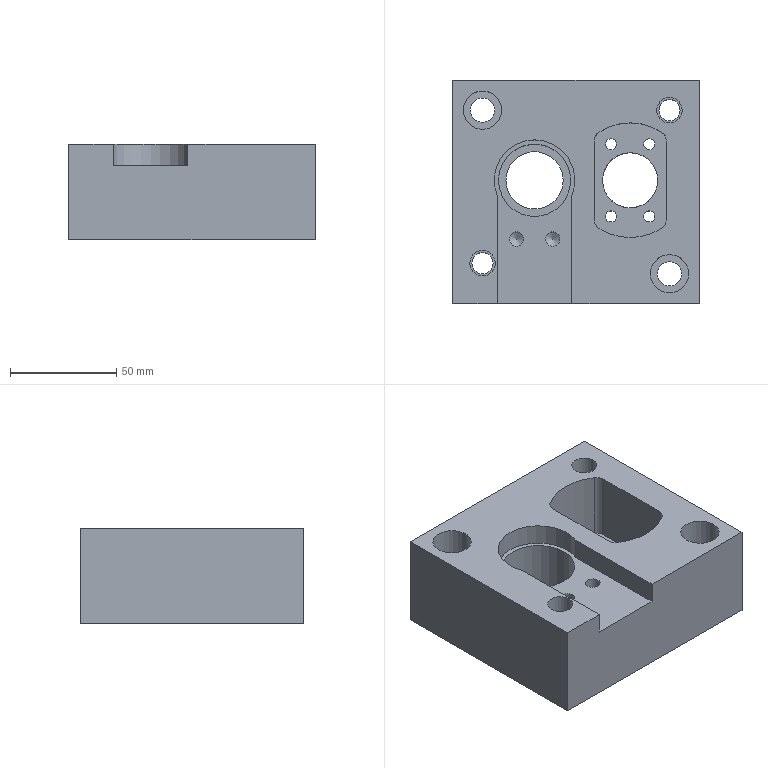Part | NX | features 26 2 | 1 solid | 43 faces | box 116 x 105 x 45 mm | volume 404154 mm3 | cylinder 24 | plane 17 | cone 2 | commonest cylinder face diameters 5.2 x4 10 x4 6.8 x2 10.001 x2 11.5 x2 12 x2
STEP:
#1=CARTESIAN_POINT('',(1383.,0.,-108.));
#2=VERTEX_POINT('',#1);
#3=CARTESIAN_POINT('',(1366.,0.,-108.));
#4=DIRECTION('',(0.,0.,1.));
#5=DIRECTION('',(1.,0.,0.));
#6=AXIS2_PLACEMENT_3D('',#3,#4,#5);
#7=CIRCLE('',#6,17.);
#8=EDGE_CURVE('',#2,#2,#7,.T.);
#9=ORIENTED_EDGE('',*,*,#8,.F.);
#10=EDGE_LOOP('',(#9));
#11=FACE_BOUND('',#10,.T.);
#12=CARTESIAN_POINT('',(1383.,0.,-78.));
#13=VERTEX_POINT('',#12);
#14=CARTESIAN_POINT('',(1366.,0.,-78.));
#15=DIRECTION('',(0.,0.,-1.));
#16=DIRECTION('',(1.,0.,0.));
#17=AXIS2_PLACEMENT_3D('',#14,#15,#16);
#18=CIRCLE('',#17,17.);
#19=EDGE_CURVE('',#13,#13,#18,.T.);
#20=ORIENTED_EDGE('',*,*,#19,.F.);
#21=EDGE_LOOP('',(#20));
#22=FACE_BOUND('',#21,.T.);
#23=CARTESIAN_POINT('',(1366.,0.,512.));
#24=DIRECTION('',(0.,0.,-1.));
#25=DIRECTION('',(1.,0.,0.));
#26=AXIS2_PLACEMENT_3D('',#23,#24,#25);
#27=CYLINDRICAL_SURFACE('',#26,17.);
#28=ADVANCED_FACE('',(#11,#22),#27,.F.);
#29=CARTESIAN_POINT('',(1383.6,-7.158,-68.));
#30=VERTEX_POINT('',#29);
#31=CARTESIAN_POINT('',(1348.4,-7.158,-68.));
#32=VERTEX_POINT('',#31);
#33=CARTESIAN_POINT('',(1366.,0.,-68.));
#34=DIRECTION('',(0.,0.,1.));
#35=DIRECTION('',(-1.,0.,0.));
#36=AXIS2_PLACEMENT_3D('',#33,#34,#35);
#37=CIRCLE('',#36,19.);
#38=EDGE_CURVE('',#30,#32,#37,.T.);
#39=ORIENTED_EDGE('',*,*,#38,.F.);
#40=CARTESIAN_POINT('',(1383.6,-58.,-68.));
#41=VERTEX_POINT('',#40);
#42=CARTESIAN_POINT('',(1383.6,206.,-68.));
#43=DIRECTION('',(0.,1.,0.));
#44=VECTOR('',#43,1000.);
#45=LINE('',#42,#44);
#46=EDGE_CURVE('',#41,#30,#45,.T.);
#47=ORIENTED_EDGE('',*,*,#46,.F.);
#48=CARTESIAN_POINT('',(1443.5,-58.,-68.));
#49=VERTEX_POINT('',#48);
#50=CARTESIAN_POINT('',(1366.,-58.,-68.));
#51=DIRECTION('',(1.,0.,0.));
#52=VECTOR('',#51,1000.);
#53=LINE('',#50,#52);
#54=EDGE_CURVE('',#41,#49,#53,.T.);
#55=ORIENTED_EDGE('',*,*,#54,.T.);
#56=CARTESIAN_POINT('',(1443.5,47.,-68.));
#57=VERTEX_POINT('',#56);
#58=CARTESIAN_POINT('',(1443.5,0.,-68.));
#59=DIRECTION('',(0.,1.,0.));
#60=VECTOR('',#59,1000.);
#61=LINE('',#58,#60);
#62=EDGE_CURVE('',#49,#57,#61,.T.);
#63=ORIENTED_EDGE('',*,*,#62,.T.);
#64=CARTESIAN_POINT('',(1327.5,47.,-68.));
#65=VERTEX_POINT('',#64);
#66=CARTESIAN_POINT('',(1366.,47.,-68.));
#67=DIRECTION('',(-1.,0.,0.));
#68=VECTOR('',#67,1000.);
#69=LINE('',#66,#68);
#70=EDGE_CURVE('',#57,#65,#69,.T.);
#71=ORIENTED_EDGE('',*,*,#70,.T.);
#72=CARTESIAN_POINT('',(1327.5,-58.,-68.));
#73=VERTEX_POINT('',#72);
#74=CARTESIAN_POINT('',(1327.5,0.,-68.));
#75=DIRECTION('',(0.,-1.,0.));
#76=VECTOR('',#75,1000.);
#77=LINE('',#74,#76);
#78=EDGE_CURVE('',#65,#73,#77,.T.);
#79=ORIENTED_EDGE('',*,*,#78,.T.);
#80=CARTESIAN_POINT('',(1348.4,-58.,-68.));
#81=VERTEX_POINT('',#80);
#82=CARTESIAN_POINT('',(1366.,-58.,-68.));
#83=DIRECTION('',(1.,0.,0.));
#84=VECTOR('',#83,1000.);
#85=LINE('',#82,#84);
#86=EDGE_CURVE('',#73,#81,#85,.T.);
#87=ORIENTED_EDGE('',*,*,#86,.T.);
#88=CARTESIAN_POINT('',(1348.4,206.,-68.));
#89=DIRECTION('',(0.,-1.,0.));
#90=VECTOR('',#89,1000.);
#91=LINE('',#88,#90);
#92=EDGE_CURVE('',#32,#81,#91,.T.);
#93=ORIENTED_EDGE('',*,*,#92,.F.);
#94=EDGE_LOOP('',(#39,#47,#55,#63,#71,#79,#87,#93));
#95=FACE_BOUND('',#94,.T.);
#96=CARTESIAN_POINT('',(1435.5,33.,-68.));
#97=VERTEX_POINT('',#96);
#98=CARTESIAN_POINT('',(1429.5,33.,-68.));
#99=DIRECTION('',(0.,0.,-1.));
#100=DIRECTION('',(1.,0.,0.));
#101=AXIS2_PLACEMENT_3D('',#98,#99,#100);
#102=CIRCLE('',#101,6.);
#103=EDGE_CURVE('',#97,#97,#102,.T.);
#104=ORIENTED_EDGE('',*,*,#103,.T.);
#105=EDGE_LOOP('',(#104));
#106=FACE_BOUND('',#105,.T.);
#107=CARTESIAN_POINT('',(1347.5,-39.,-68.));
#108=VERTEX_POINT('',#107);
#109=CARTESIAN_POINT('',(1341.5,-39.,-68.));
#110=DIRECTION('',(0.,0.,-1.));
#111=DIRECTION('',(1.,0.,0.));
#112=AXIS2_PLACEMENT_3D('',#109,#110,#111);
#113=CIRCLE('',#112,6.);
#114=EDGE_CURVE('',#108,#108,#113,.T.);
#115=ORIENTED_EDGE('',*,*,#114,.T.);
#116=EDGE_LOOP('',(#115));
#117=FACE_BOUND('',#116,.T.);
#118=CARTESIAN_POINT('',(1332.5,33.,-68.));
#119=VERTEX_POINT('',#118);
#120=CARTESIAN_POINT('',(1341.5,33.,-68.));
#121=DIRECTION('',(0.,0.,1.));
#122=DIRECTION('',(-1.,0.,0.));
#123=AXIS2_PLACEMENT_3D('',#120,#121,#122);
#124=CIRCLE('',#123,9.);
#125=EDGE_CURVE('',#119,#119,#124,.T.);
#126=ORIENTED_EDGE('',*,*,#125,.F.);
#127=EDGE_LOOP('',(#126));
#128=FACE_BOUND('',#127,.T.);
#129=CARTESIAN_POINT('',(1420.5,-44.,-68.));
#130=VERTEX_POINT('',#129);
#131=CARTESIAN_POINT('',(1429.5,-44.,-68.));
#132=DIRECTION('',(0.,0.,1.));
#133=DIRECTION('',(-1.,0.,0.));
#134=AXIS2_PLACEMENT_3D('',#131,#132,#133);
#135=CIRCLE('',#134,9.);
#136=EDGE_CURVE('',#130,#130,#135,.T.);
#137=ORIENTED_EDGE('',*,*,#136,.F.);
#138=EDGE_LOOP('',(#137));
#139=FACE_BOUND('',#138,.T.);
#140=CARTESIAN_POINT('',(1394.,18.439,-68.));
#141=VERTEX_POINT('',#140);
#142=CARTESIAN_POINT('',(1394.,-18.439,-68.));
#143=VERTEX_POINT('',#142);
#144=CARTESIAN_POINT('',(1394.,211.,-68.));
#145=DIRECTION('',(0.,-1.,0.));
#146=VECTOR('',#145,1000.);
#147=LINE('',#144,#146);
#148=EDGE_CURVE('',#141,#143,#147,.T.);
#149=ORIENTED_EDGE('',*,*,#148,.F.);
#150=CARTESIAN_POINT('',(1396.273,22.63,-68.));
#151=VERTEX_POINT('',#150);
#152=CARTESIAN_POINT('',(1399.,18.439,-68.));
#153=DIRECTION('',(0.,0.,1.));
#154=DIRECTION('',(1.,0.,0.));
#155=AXIS2_PLACEMENT_3D('',#152,#153,#154);
#156=CIRCLE('',#155,5.);
#157=EDGE_CURVE('',#151,#141,#156,.T.);
#158=ORIENTED_EDGE('',*,*,#157,.F.);
#159=CARTESIAN_POINT('',(1425.727,22.63,-68.));
#160=VERTEX_POINT('',#159);
#161=CARTESIAN_POINT('',(1411.,0.,-68.));
#162=DIRECTION('',(0.,0.,1.));
#163=DIRECTION('',(1.,0.,0.));
#164=AXIS2_PLACEMENT_3D('',#161,#162,#163);
#165=CIRCLE('',#164,27.);
#166=EDGE_CURVE('',#160,#151,#165,.T.);
#167=ORIENTED_EDGE('',*,*,#166,.F.);
#168=CARTESIAN_POINT('',(1428.,18.439,-68.));
#169=VERTEX_POINT('',#168);
#170=CARTESIAN_POINT('',(1423.,18.439,-68.));
#171=DIRECTION('',(0.,0.,1.));
#172=DIRECTION('',(1.,0.,0.));
#173=AXIS2_PLACEMENT_3D('',#170,#171,#172);
#174=CIRCLE('',#173,5.);
#175=EDGE_CURVE('',#169,#160,#174,.T.);
#176=ORIENTED_EDGE('',*,*,#175,.F.);
#177=CARTESIAN_POINT('',(1428.,-18.439,-68.));
#178=VERTEX_POINT('',#177);
#179=CARTESIAN_POINT('',(1428.,211.,-68.));
#180=DIRECTION('',(0.,1.,0.));
#181=VECTOR('',#180,1000.);
#182=LINE('',#179,#181);
#183=EDGE_CURVE('',#178,#169,#182,.T.);
#184=ORIENTED_EDGE('',*,*,#183,.F.);
#185=CARTESIAN_POINT('',(1425.727,-22.63,-68.));
#186=VERTEX_POINT('',#185);
#187=CARTESIAN_POINT('',(1423.,-18.439,-68.));
#188=DIRECTION('',(0.,0.,1.));
#189=DIRECTION('',(1.,0.,0.));
#190=AXIS2_PLACEMENT_3D('',#187,#188,#189);
#191=CIRCLE('',#190,5.);
#192=EDGE_CURVE('',#186,#178,#191,.T.);
#193=ORIENTED_EDGE('',*,*,#192,.F.);
#194=CARTESIAN_POINT('',(1396.273,-22.63,-68.));
#195=VERTEX_POINT('',#194);
#196=CARTESIAN_POINT('',(1411.,0.,-68.));
#197=DIRECTION('',(0.,0.,1.));
#198=DIRECTION('',(1.,0.,0.));
#199=AXIS2_PLACEMENT_3D('',#196,#197,#198);
#200=CIRCLE('',#199,27.);
#201=EDGE_CURVE('',#195,#186,#200,.T.);
#202=ORIENTED_EDGE('',*,*,#201,.F.);
#203=CARTESIAN_POINT('',(1399.,-18.439,-68.));
#204=DIRECTION('',(0.,0.,1.));
#205=DIRECTION('',(1.,0.,0.));
#206=AXIS2_PLACEMENT_3D('',#203,#204,#205);
#207=CIRCLE('',#206,5.);
#208=EDGE_CURVE('',#143,#195,#207,.T.);
#209=ORIENTED_EDGE('',*,*,#208,.F.);
#210=EDGE_LOOP('',(#149,#158,#167,#176,#184,#193,#202,#209));
#211=FACE_BOUND('',#210,.T.);
#212=CARTESIAN_POINT('',(2530.5,206.,-68.));
#213=DIRECTION('',(0.,0.,-1.));
#214=DIRECTION('',(1.,0.,0.));
#215=AXIS2_PLACEMENT_3D('',#212,#213,#214);
#216=PLANE('',#215);
#217=ADVANCED_FACE('',(#95,#106,#117,#128,#139,#211),#216,.F.);
#218=CARTESIAN_POINT('',(1327.5,-58.,-113.));
#219=VERTEX_POINT('',#218);
#220=CARTESIAN_POINT('',(1327.5,-58.,-123.5));
#221=DIRECTION('',(0.,0.,1.));
#222=VECTOR('',#221,1000.);
#223=LINE('',#220,#222);
#224=EDGE_CURVE('',#219,#73,#223,.T.);
#225=ORIENTED_EDGE('',*,*,#224,.T.);
#226=ORIENTED_EDGE('',*,*,#78,.F.);
#227=CARTESIAN_POINT('',(1327.5,47.,-113.));
#228=VERTEX_POINT('',#227);
#229=CARTESIAN_POINT('',(1327.5,47.,-123.5));
#230=DIRECTION('',(0.,0.,1.));
#231=VECTOR('',#230,1000.);
#232=LINE('',#229,#231);
#233=EDGE_CURVE('',#228,#65,#232,.T.);
#234=ORIENTED_EDGE('',*,*,#233,.F.);
#235=CARTESIAN_POINT('',(1327.5,0.,-113.));
#236=DIRECTION('',(0.,1.,0.));
#237=VECTOR('',#236,1000.);
#238=LINE('',#235,#237);
#239=EDGE_CURVE('',#219,#228,#238,.T.);
#240=ORIENTED_EDGE('',*,*,#239,.F.);
#241=EDGE_LOOP('',(#225,#226,#234,#240));
#242=FACE_BOUND('',#241,.T.);
#243=CARTESIAN_POINT('',(1327.5,0.,-123.5));
#244=DIRECTION('',(-1.,0.,0.));
#245=DIRECTION('',(0.,0.,-1.));
#246=AXIS2_PLACEMENT_3D('',#243,#244,#245);
#247=PLANE('',#246);
#248=ADVANCED_FACE('',(#242),#247,.T.);
#249=ORIENTED_EDGE('',*,*,#233,.T.);
#250=ORIENTED_EDGE('',*,*,#70,.F.);
#251=CARTESIAN_POINT('',(1443.5,47.,-113.));
#252=VERTEX_POINT('',#251);
#253=CARTESIAN_POINT('',(1443.5,47.,-123.5));
#254=DIRECTION('',(0.,0.,1.));
#255=VECTOR('',#254,1000.);
#256=LINE('',#253,#255);
#257=EDGE_CURVE('',#252,#57,#256,.T.);
#258=ORIENTED_EDGE('',*,*,#257,.F.);
#259=CARTESIAN_POINT('',(1366.,47.,-113.));
#260=DIRECTION('',(1.,0.,0.));
#261=VECTOR('',#260,1000.);
#262=LINE('',#259,#261);
#263=EDGE_CURVE('',#228,#252,#262,.T.);
#264=ORIENTED_EDGE('',*,*,#263,.F.);
#265=EDGE_LOOP('',(#249,#250,#258,#264));
#266=FACE_BOUND('',#265,.T.);
#267=CARTESIAN_POINT('',(1366.,47.,-123.5));
#268=DIRECTION('',(0.,1.,0.));
#269=DIRECTION('',(0.,0.,1.));
#270=AXIS2_PLACEMENT_3D('',#267,#268,#269);
#271=PLANE('',#270);
#272=ADVANCED_FACE('',(#266),#271,.T.);
#273=ORIENTED_EDGE('',*,*,#257,.T.);
#274=ORIENTED_EDGE('',*,*,#62,.F.);
#275=CARTESIAN_POINT('',(1443.5,-58.,-113.));
#276=VERTEX_POINT('',#275);
#277=CARTESIAN_POINT('',(1443.5,-58.,-123.5));
#278=DIRECTION('',(0.,0.,1.));
#279=VECTOR('',#278,1000.);
#280=LINE('',#277,#279);
#281=EDGE_CURVE('',#276,#49,#280,.T.);
#282=ORIENTED_EDGE('',*,*,#281,.F.);
#283=CARTESIAN_POINT('',(1443.5,0.,-113.));
#284=DIRECTION('',(0.,-1.,0.));
#285=VECTOR('',#284,1000.);
#286=LINE('',#283,#285);
#287=EDGE_CURVE('',#252,#276,#286,.T.);
#288=ORIENTED_EDGE('',*,*,#287,.F.);
#289=EDGE_LOOP('',(#273,#274,#282,#288));
#290=FACE_BOUND('',#289,.T.);
#291=CARTESIAN_POINT('',(1443.5,0.,-123.5));
#292=DIRECTION('',(1.,0.,0.));
#293=DIRECTION('',(0.,0.,1.));
#294=AXIS2_PLACEMENT_3D('',#291,#292,#293);
#295=PLANE('',#294);
#296=ADVANCED_FACE('',(#290),#295,.T.);
#297=CARTESIAN_POINT('',(1383.6,-58.,-78.));
#298=VERTEX_POINT('',#297);
#299=CARTESIAN_POINT('',(1383.6,-58.,-123.5));
#300=DIRECTION('',(0.,0.,-1.));
#301=VECTOR('',#300,1000.);
#302=LINE('',#299,#301);
#303=EDGE_CURVE('',#41,#298,#302,.T.);
#304=ORIENTED_EDGE('',*,*,#303,.T.);
#305=CARTESIAN_POINT('',(1348.4,-58.,-78.));
#306=VERTEX_POINT('',#305);
#307=CARTESIAN_POINT('',(1366.,-58.,-78.));
#308=DIRECTION('',(-1.,0.,0.));
#309=VECTOR('',#308,1000.);
#310=LINE('',#307,#309);
#311=EDGE_CURVE('',#298,#306,#310,.T.);
#312=ORIENTED_EDGE('',*,*,#311,.T.);
#313=CARTESIAN_POINT('',(1348.4,-58.,-58.));
#314=DIRECTION('',(0.,0.,-1.));
#315=VECTOR('',#314,1000.);
#316=LINE('',#313,#315);
#317=EDGE_CURVE('',#81,#306,#316,.T.);
#318=ORIENTED_EDGE('',*,*,#317,.F.);
#319=ORIENTED_EDGE('',*,*,#86,.F.);
#320=ORIENTED_EDGE('',*,*,#224,.F.);
#321=CARTESIAN_POINT('',(1366.,-58.,-113.));
#322=DIRECTION('',(-1.,0.,0.));
#323=VECTOR('',#322,1000.);
#324=LINE('',#321,#323);
#325=EDGE_CURVE('',#276,#219,#324,.T.);
#326=ORIENTED_EDGE('',*,*,#325,.F.);
#327=ORIENTED_EDGE('',*,*,#281,.T.);
#328=ORIENTED_EDGE('',*,*,#54,.F.);
#329=EDGE_LOOP('',(#304,#312,#318,#319,#320,#326,#327,#328));
#330=FACE_BOUND('',#329,.T.);
#331=CARTESIAN_POINT('',(1366.,-58.,-123.5));
#332=DIRECTION('',(0.,-1.,0.));
#333=DIRECTION('',(0.,0.,-1.));
#334=AXIS2_PLACEMENT_3D('',#331,#332,#333);
#335=PLANE('',#334);
#336=ADVANCED_FACE('',(#330),#335,.T.);
#337=CARTESIAN_POINT('',(1336.499,-39.,-88.5));
#338=VERTEX_POINT('',#337);
#339=CARTESIAN_POINT('',(1341.5,-39.,-88.5));
#340=DIRECTION('',(0.,0.,1.));
#341=DIRECTION('',(-1.,0.,0.));
#342=AXIS2_PLACEMENT_3D('',#339,#340,#341);
#343=CIRCLE('',#342,5.);
#344=EDGE_CURVE('',#338,#338,#343,.T.);
#345=ORIENTED_EDGE('',*,*,#344,.T.);
#346=EDGE_LOOP('',(#345));
#347=FACE_BOUND('',#346,.T.);
#348=CARTESIAN_POINT('',(1336.499,-39.,-113.));
#349=VERTEX_POINT('',#348);
#350=CARTESIAN_POINT('',(1341.5,-39.,-113.));
#351=DIRECTION('',(0.,0.,-1.));
#352=DIRECTION('',(-1.,0.,0.));
#353=AXIS2_PLACEMENT_3D('',#350,#351,#352);
#354=CIRCLE('',#353,5.);
#355=EDGE_CURVE('',#349,#349,#354,.T.);
#356=ORIENTED_EDGE('',*,*,#355,.T.);
#357=EDGE_LOOP('',(#356));
#358=FACE_BOUND('',#357,.T.);
#359=CARTESIAN_POINT('',(1341.5,-39.,541.5));
#360=DIRECTION('',(0.,0.,-1.));
#361=DIRECTION('',(1.,0.,0.));
#362=AXIS2_PLACEMENT_3D('',#359,#360,#361);
#363=CYLINDRICAL_SURFACE('',#362,5.);
#364=ADVANCED_FACE('',(#347,#358),#363,.F.);
#365=CARTESIAN_POINT('',(1424.499,33.,-88.5));
#366=VERTEX_POINT('',#365);
#367=CARTESIAN_POINT('',(1429.5,33.,-88.5));
#368=DIRECTION('',(0.,0.,1.));
#369=DIRECTION('',(-1.,0.,0.));
#370=AXIS2_PLACEMENT_3D('',#367,#368,#369);
#371=CIRCLE('',#370,5.);
#372=EDGE_CURVE('',#366,#366,#371,.T.);
#373=ORIENTED_EDGE('',*,*,#372,.T.);
#374=EDGE_LOOP('',(#373));
#375=FACE_BOUND('',#374,.T.);
#376=CARTESIAN_POINT('',(1424.499,33.,-113.));
#377=VERTEX_POINT('',#376);
#378=CARTESIAN_POINT('',(1429.5,33.,-113.));
#379=DIRECTION('',(0.,0.,-1.));
#380=DIRECTION('',(-1.,0.,0.));
#381=AXIS2_PLACEMENT_3D('',#378,#379,#380);
#382=CIRCLE('',#381,5.);
#383=EDGE_CURVE('',#377,#377,#382,.T.);
#384=ORIENTED_EDGE('',*,*,#383,.T.);
#385=EDGE_LOOP('',(#384));
#386=FACE_BOUND('',#385,.T.);
#387=CARTESIAN_POINT('',(1429.5,33.,541.5));
#388=DIRECTION('',(0.,0.,-1.));
#389=DIRECTION('',(1.,0.,0.));
#390=AXIS2_PLACEMENT_3D('',#387,#388,#389);
#391=CYLINDRICAL_SURFACE('',#390,5.);
#392=ADVANCED_FACE('',(#375,#386),#391,.F.);
#393=CARTESIAN_POINT('',(1335.75,33.,-88.5));
#394=VERTEX_POINT('',#393);
#395=CARTESIAN_POINT('',(1341.5,33.,-88.5));
#396=DIRECTION('',(0.,0.,1.));
#397=DIRECTION('',(-1.,0.,0.));
#398=AXIS2_PLACEMENT_3D('',#395,#396,#397);
#399=CIRCLE('',#398,5.75);
#400=EDGE_CURVE('',#394,#394,#399,.T.);
#401=ORIENTED_EDGE('',*,*,#400,.T.);
#402=EDGE_LOOP('',(#401));
#403=FACE_BOUND('',#402,.T.);
#404=CARTESIAN_POINT('',(1335.75,33.,-113.));
#405=VERTEX_POINT('',#404);
#406=CARTESIAN_POINT('',(1341.5,33.,-113.));
#407=DIRECTION('',(0.,0.,-1.));
#408=DIRECTION('',(-1.,0.,0.));
#409=AXIS2_PLACEMENT_3D('',#406,#407,#408);
#410=CIRCLE('',#409,5.75);
#411=EDGE_CURVE('',#405,#405,#410,.T.);
#412=ORIENTED_EDGE('',*,*,#411,.T.);
#413=EDGE_LOOP('',(#412));
#414=FACE_BOUND('',#413,.T.);
#415=CARTESIAN_POINT('',(1341.5,33.,-66.5));
#416=DIRECTION('',(0.,0.,-1.));
#417=DIRECTION('',(-1.,0.,0.));
#418=AXIS2_PLACEMENT_3D('',#415,#416,#417);
#419=CYLINDRICAL_SURFACE('',#418,5.75);
#420=ADVANCED_FACE('',(#403,#414),#419,.F.);
#421=CARTESIAN_POINT('',(1423.75,-44.,-88.5));
#422=VERTEX_POINT('',#421);
#423=CARTESIAN_POINT('',(1429.5,-44.,-88.5));
#424=DIRECTION('',(0.,0.,1.));
#425=DIRECTION('',(-1.,0.,0.));
#426=AXIS2_PLACEMENT_3D('',#423,#424,#425);
#427=CIRCLE('',#426,5.75);
#428=EDGE_CURVE('',#422,#422,#427,.T.);
#429=ORIENTED_EDGE('',*,*,#428,.T.);
#430=EDGE_LOOP('',(#429));
#431=FACE_BOUND('',#430,.T.);
#432=CARTESIAN_POINT('',(1423.75,-44.,-113.));
#433=VERTEX_POINT('',#432);
#434=CARTESIAN_POINT('',(1429.5,-44.,-113.));
#435=DIRECTION('',(0.,0.,-1.));
#436=DIRECTION('',(-1.,0.,0.));
#437=AXIS2_PLACEMENT_3D('',#434,#435,#436);
#438=CIRCLE('',#437,5.75);
#439=EDGE_CURVE('',#433,#433,#438,.T.);
#440=ORIENTED_EDGE('',*,*,#439,.T.);
#441=EDGE_LOOP('',(#440));
#442=FACE_BOUND('',#441,.T.);
#443=CARTESIAN_POINT('',(1429.5,-44.,-66.5));
#444=DIRECTION('',(0.,0.,-1.));
#445=DIRECTION('',(-1.,0.,0.));
#446=AXIS2_PLACEMENT_3D('',#443,#444,#445);
#447=CYLINDRICAL_SURFACE('',#446,5.75);
#448=ADVANCED_FACE('',(#431,#442),#447,.F.);
#449=CARTESIAN_POINT('',(1379.5,0.,-108.));
#450=VERTEX_POINT('',#449);
#451=CARTESIAN_POINT('',(1366.,0.,-108.));
#452=DIRECTION('',(0.,0.,1.));
#453=DIRECTION('',(1.,0.,0.));
#454=AXIS2_PLACEMENT_3D('',#451,#452,#453);
#455=CIRCLE('',#454,13.5);
#456=EDGE_CURVE('',#450,#450,#455,.T.);
#457=ORIENTED_EDGE('',*,*,#456,.T.);
#458=EDGE_LOOP('',(#457));
#459=FACE_BOUND('',#458,.T.);
#460=CARTESIAN_POINT('',(1352.5,0.,-113.));
#461=VERTEX_POINT('',#460);
#462=CARTESIAN_POINT('',(1366.,0.,-113.));
#463=DIRECTION('',(0.,0.,-1.));
#464=DIRECTION('',(-1.,0.,0.));
#465=AXIS2_PLACEMENT_3D('',#462,#463,#464);
#466=CIRCLE('',#465,13.5);
#467=EDGE_CURVE('',#461,#461,#466,.T.);
#468=ORIENTED_EDGE('',*,*,#467,.T.);
#469=EDGE_LOOP('',(#468));
#470=FACE_BOUND('',#469,.T.);
#471=CARTESIAN_POINT('',(1366.,0.,542.));
#472=DIRECTION('',(0.,0.,-1.));
#473=DIRECTION('',(1.,0.,0.));
#474=AXIS2_PLACEMENT_3D('',#471,#472,#473);
#475=CYLINDRICAL_SURFACE('',#474,13.5);
#476=ADVANCED_FACE('',(#459,#470),#475,.F.);
#477=CARTESIAN_POINT('',(1423.5,33.,-88.5));
#478=VERTEX_POINT('',#477);
#479=CARTESIAN_POINT('',(1429.5,33.,-88.5));
#480=DIRECTION('',(0.,0.,-1.));
#481=DIRECTION('',(-1.,0.,0.));
#482=AXIS2_PLACEMENT_3D('',#479,#480,#481);
#483=CIRCLE('',#482,6.);
#484=EDGE_CURVE('',#478,#478,#483,.T.);
#485=ORIENTED_EDGE('',*,*,#484,.T.);
#486=EDGE_LOOP('',(#485));
#487=FACE_BOUND('',#486,.T.);
#488=ORIENTED_EDGE('',*,*,#103,.F.);
#489=EDGE_LOOP('',(#488));
#490=FACE_BOUND('',#489,.T.);
#491=CARTESIAN_POINT('',(1429.5,33.,541.5));
#492=DIRECTION('',(0.,0.,-1.));
#493=DIRECTION('',(1.,0.,0.));
#494=AXIS2_PLACEMENT_3D('',#491,#492,#493);
#495=CYLINDRICAL_SURFACE('',#494,6.);
#496=ADVANCED_FACE('',(#487,#490),#495,.F.);
#497=ORIENTED_EDGE('',*,*,#114,.F.);
#498=EDGE_LOOP('',(#497));
#499=FACE_BOUND('',#498,.T.);
#500=CARTESIAN_POINT('',(1335.5,-39.,-88.5));
#501=VERTEX_POINT('',#500);
#502=CARTESIAN_POINT('',(1341.5,-39.,-88.5));
#503=DIRECTION('',(0.,0.,-1.));
#504=DIRECTION('',(-1.,0.,0.));
#505=AXIS2_PLACEMENT_3D('',#502,#503,#504);
#506=CIRCLE('',#505,6.);
#507=EDGE_CURVE('',#501,#501,#506,.T.);
#508=ORIENTED_EDGE('',*,*,#507,.T.);
#509=EDGE_LOOP('',(#508));
#510=FACE_BOUND('',#509,.T.);
#511=CARTESIAN_POINT('',(1341.5,-39.,541.5));
#512=DIRECTION('',(0.,0.,-1.));
#513=DIRECTION('',(1.,0.,0.));
#514=AXIS2_PLACEMENT_3D('',#511,#512,#513);
#515=CYLINDRICAL_SURFACE('',#514,6.);
#516=ADVANCED_FACE('',(#499,#510),#515,.F.);
#517=CARTESIAN_POINT('',(1332.5,33.,-88.5));
#518=VERTEX_POINT('',#517);
#519=CARTESIAN_POINT('',(1341.5,33.,-88.5));
#520=DIRECTION('',(0.,0.,1.));
#521=DIRECTION('',(-1.,0.,0.));
#522=AXIS2_PLACEMENT_3D('',#519,#520,#521);
#523=CIRCLE('',#522,9.);
#524=EDGE_CURVE('',#518,#518,#523,.T.);
#525=ORIENTED_EDGE('',*,*,#524,.F.);
#526=EDGE_LOOP('',(#525));
#527=FACE_BOUND('',#526,.T.);
#528=ORIENTED_EDGE('',*,*,#125,.T.);
#529=EDGE_LOOP('',(#528));
#530=FACE_BOUND('',#529,.T.);
#531=CARTESIAN_POINT('',(1341.5,33.,-68.5));
#532=DIRECTION('',(0.,0.,-1.));
#533=DIRECTION('',(-1.,0.,0.));
#534=AXIS2_PLACEMENT_3D('',#531,#532,#533);
#535=CYLINDRICAL_SURFACE('',#534,9.);
#536=ADVANCED_FACE('',(#527,#530),#535,.F.);
#537=CARTESIAN_POINT('',(1420.5,-44.,-88.5));
#538=VERTEX_POINT('',#537);
#539=CARTESIAN_POINT('',(1429.5,-44.,-88.5));
#540=DIRECTION('',(0.,0.,1.));
#541=DIRECTION('',(-1.,0.,0.));
#542=AXIS2_PLACEMENT_3D('',#539,#540,#541);
#543=CIRCLE('',#542,9.);
#544=EDGE_CURVE('',#538,#538,#543,.T.);
#545=ORIENTED_EDGE('',*,*,#544,.F.);
#546=EDGE_LOOP('',(#545));
#547=FACE_BOUND('',#546,.T.);
#548=ORIENTED_EDGE('',*,*,#136,.T.);
#549=EDGE_LOOP('',(#548));
#550=FACE_BOUND('',#549,.T.);
#551=CARTESIAN_POINT('',(1429.5,-44.,-68.5));
#552=DIRECTION('',(0.,0.,-1.));
#553=DIRECTION('',(-1.,0.,0.));
#554=AXIS2_PLACEMENT_3D('',#551,#552,#553);
#555=CYLINDRICAL_SURFACE('',#554,9.);
#556=ADVANCED_FACE('',(#547,#550),#555,.F.);
#557=ORIENTED_EDGE('',*,*,#544,.T.);
#558=EDGE_LOOP('',(#557));
#559=FACE_BOUND('',#558,.T.);
#560=ORIENTED_EDGE('',*,*,#428,.F.);
#561=EDGE_LOOP('',(#560));
#562=FACE_BOUND('',#561,.T.);
#563=CARTESIAN_POINT('',(1372.5,-2.,-88.5));
#564=DIRECTION('',(0.,0.,-1.));
#565=DIRECTION('',(1.,0.,0.));
#566=AXIS2_PLACEMENT_3D('',#563,#564,#565);
#567=PLANE('',#566);
#568=ADVANCED_FACE('',(#559,#562),#567,.F.);
#569=ORIENTED_EDGE('',*,*,#484,.F.);
#570=EDGE_LOOP('',(#569));
#571=FACE_BOUND('',#570,.T.);
#572=ORIENTED_EDGE('',*,*,#372,.F.);
#573=EDGE_LOOP('',(#572));
#574=FACE_BOUND('',#573,.T.);
#575=CARTESIAN_POINT('',(1372.5,33.,-88.5));
#576=DIRECTION('',(0.,0.,-1.));
#577=DIRECTION('',(1.,0.,0.));
#578=AXIS2_PLACEMENT_3D('',#575,#576,#577);
#579=PLANE('',#578);
#580=ADVANCED_FACE('',(#571,#574),#579,.F.);
#581=ORIENTED_EDGE('',*,*,#507,.F.);
#582=EDGE_LOOP('',(#581));
#583=FACE_BOUND('',#582,.T.);
#584=ORIENTED_EDGE('',*,*,#344,.F.);
#585=EDGE_LOOP('',(#584));
#586=FACE_BOUND('',#585,.T.);
#587=CARTESIAN_POINT('',(1341.5,3.,-88.5));
#588=DIRECTION('',(0.,0.,-1.));
#589=DIRECTION('',(1.,0.,0.));
#590=AXIS2_PLACEMENT_3D('',#587,#588,#589);
#591=PLANE('',#590);
#592=ADVANCED_FACE('',(#583,#586),#591,.F.);
#593=ORIENTED_EDGE('',*,*,#8,.T.);
#594=EDGE_LOOP('',(#593));
#595=FACE_BOUND('',#594,.T.);
#596=ORIENTED_EDGE('',*,*,#456,.F.);
#597=EDGE_LOOP('',(#596));
#598=FACE_BOUND('',#597,.T.);
#599=CARTESIAN_POINT('',(1366.,0.,-108.));
#600=DIRECTION('',(0.,0.,1.));
#601=DIRECTION('',(-1.,0.,0.));
#602=AXIS2_PLACEMENT_3D('',#599,#600,#601);
#603=PLANE('',#602);
#604=ADVANCED_FACE('',(#595,#598),#603,.T.);
#605=ORIENTED_EDGE('',*,*,#524,.T.);
#606=EDGE_LOOP('',(#605));
#607=FACE_BOUND('',#606,.T.);
#608=ORIENTED_EDGE('',*,*,#400,.F.);
#609=EDGE_LOOP('',(#608));
#610=FACE_BOUND('',#609,.T.);
#611=CARTESIAN_POINT('',(1341.5,33.,-88.5));
#612=DIRECTION('',(0.,0.,-1.));
#613=DIRECTION('',(1.,0.,0.));
#614=AXIS2_PLACEMENT_3D('',#611,#612,#613);
#615=PLANE('',#614);
#616=ADVANCED_FACE('',(#607,#610),#615,.F.);
#617=CARTESIAN_POINT('',(1399.4,17.,-113.));
#618=VERTEX_POINT('',#617);
#619=CARTESIAN_POINT('',(1402.,17.,-113.));
#620=DIRECTION('',(0.,0.,-1.));
#621=DIRECTION('',(-1.,0.,0.));
#622=AXIS2_PLACEMENT_3D('',#619,#620,#621);
#623=CIRCLE('',#622,2.6);
#624=EDGE_CURVE('',#618,#618,#623,.T.);
#625=ORIENTED_EDGE('',*,*,#624,.F.);
#626=EDGE_LOOP('',(#625));
#627=FACE_BOUND('',#626,.T.);
#628=CARTESIAN_POINT('',(1399.4,-17.,-113.));
#629=VERTEX_POINT('',#628);
#630=CARTESIAN_POINT('',(1402.,-17.,-113.));
#631=DIRECTION('',(0.,0.,-1.));
#632=DIRECTION('',(-1.,0.,0.));
#633=AXIS2_PLACEMENT_3D('',#630,#631,#632);
#634=CIRCLE('',#633,2.6);
#635=EDGE_CURVE('',#629,#629,#634,.T.);
#636=ORIENTED_EDGE('',*,*,#635,.F.);
#637=EDGE_LOOP('',(#636));
#638=FACE_BOUND('',#637,.T.);
#639=CARTESIAN_POINT('',(1417.4,17.,-113.));
#640=VERTEX_POINT('',#639);
#641=CARTESIAN_POINT('',(1420.,17.,-113.));
#642=DIRECTION('',(0.,0.,-1.));
#643=DIRECTION('',(-1.,0.,0.));
#644=AXIS2_PLACEMENT_3D('',#641,#642,#643);
#645=CIRCLE('',#644,2.6);
#646=EDGE_CURVE('',#640,#640,#645,.T.);
#647=ORIENTED_EDGE('',*,*,#646,.F.);
#648=EDGE_LOOP('',(#647));
#649=FACE_BOUND('',#648,.T.);
#650=CARTESIAN_POINT('',(1417.4,-17.,-113.));
#651=VERTEX_POINT('',#650);
#652=CARTESIAN_POINT('',(1420.,-17.,-113.));
#653=DIRECTION('',(0.,0.,-1.));
#654=DIRECTION('',(-1.,0.,0.));
#655=AXIS2_PLACEMENT_3D('',#652,#653,#654);
#656=CIRCLE('',#655,2.6);
#657=EDGE_CURVE('',#651,#651,#656,.T.);
#658=ORIENTED_EDGE('',*,*,#657,.F.);
#659=EDGE_LOOP('',(#658));
#660=FACE_BOUND('',#659,.T.);
#661=CARTESIAN_POINT('',(1424.,0.,-113.));
#662=VERTEX_POINT('',#661);
#663=CARTESIAN_POINT('',(1411.,0.,-113.));
#664=DIRECTION('',(0.,0.,1.));
#665=DIRECTION('',(1.,0.,0.));
#666=AXIS2_PLACEMENT_3D('',#663,#664,#665);
#667=CIRCLE('',#666,13.);
#668=EDGE_CURVE('',#662,#662,#667,.T.);
#669=ORIENTED_EDGE('',*,*,#668,.T.);
#670=EDGE_LOOP('',(#669));
#671=FACE_BOUND('',#670,.T.);
#672=ORIENTED_EDGE('',*,*,#239,.T.);
#673=ORIENTED_EDGE('',*,*,#263,.T.);
#674=ORIENTED_EDGE('',*,*,#287,.T.);
#675=ORIENTED_EDGE('',*,*,#325,.T.);
#676=EDGE_LOOP('',(#672,#673,#674,#675));
#677=FACE_BOUND('',#676,.T.);
#678=ORIENTED_EDGE('',*,*,#383,.F.);
#679=EDGE_LOOP('',(#678));
#680=FACE_BOUND('',#679,.T.);
#681=ORIENTED_EDGE('',*,*,#439,.F.);
#682=EDGE_LOOP('',(#681));
#683=FACE_BOUND('',#682,.T.);
#684=ORIENTED_EDGE('',*,*,#467,.F.);
#685=EDGE_LOOP('',(#684));
#686=FACE_BOUND('',#685,.T.);
#687=ORIENTED_EDGE('',*,*,#411,.F.);
#688=EDGE_LOOP('',(#687));
#689=FACE_BOUND('',#688,.T.);
#690=ORIENTED_EDGE('',*,*,#355,.F.);
#691=EDGE_LOOP('',(#690));
#692=FACE_BOUND('',#691,.T.);
#693=CARTESIAN_POINT('',(2596.,-3.,-113.));
#694=DIRECTION('',(0.,0.,-1.));
#695=DIRECTION('',(-1.,0.,0.));
#696=AXIS2_PLACEMENT_3D('',#693,#694,#695);
#697=PLANE('',#696);
#698=ADVANCED_FACE('',(#627,#638,#649,#660,#671,#677,#680,#683,#686,#689,#692),#697,.T.);
#699=CARTESIAN_POINT('',(1411.,13.,-100.));
#700=VERTEX_POINT('',#699);
#701=CARTESIAN_POINT('',(1411.,0.,-100.));
#702=DIRECTION('',(0.,0.,-1.));
#703=DIRECTION('',(0.,1.,0.));
#704=AXIS2_PLACEMENT_3D('',#701,#702,#703);
#705=CIRCLE('',#704,13.);
#706=EDGE_CURVE('',#700,#700,#705,.T.);
#707=ORIENTED_EDGE('',*,*,#706,.F.);
#708=EDGE_LOOP('',(#707));
#709=FACE_BOUND('',#708,.T.);
#710=ORIENTED_EDGE('',*,*,#668,.F.);
#711=EDGE_LOOP('',(#710));
#712=FACE_BOUND('',#711,.T.);
#713=CARTESIAN_POINT('',(1411.,0.,-95.5));
#714=DIRECTION('',(0.,0.,1.));
#715=DIRECTION('',(-1.,0.,0.));
#716=AXIS2_PLACEMENT_3D('',#713,#714,#715);
#717=CYLINDRICAL_SURFACE('',#716,13.);
#718=ADVANCED_FACE('',(#709,#712),#717,.F.);
#719=ORIENTED_EDGE('',*,*,#201,.T.);
#720=CARTESIAN_POINT('',(1425.727,-22.63,-100.));
#721=VERTEX_POINT('',#720);
#722=CARTESIAN_POINT('',(1425.727,-22.63,-95.5));
#723=DIRECTION('',(0.,0.,1.));
#724=VECTOR('',#723,1000.);
#725=LINE('',#722,#724);
#726=EDGE_CURVE('',#721,#186,#725,.T.);
#727=ORIENTED_EDGE('',*,*,#726,.F.);
#728=CARTESIAN_POINT('',(1396.273,-22.63,-100.));
#729=VERTEX_POINT('',#728);
#730=CARTESIAN_POINT('',(1411.,0.,-100.));
#731=DIRECTION('',(0.,0.,-1.));
#732=DIRECTION('',(0.,1.,0.));
#733=AXIS2_PLACEMENT_3D('',#730,#731,#732);
#734=CIRCLE('',#733,27.);
#735=EDGE_CURVE('',#721,#729,#734,.T.);
#736=ORIENTED_EDGE('',*,*,#735,.T.);
#737=CARTESIAN_POINT('',(1396.273,-22.63,-95.5));
#738=DIRECTION('',(0.,0.,-1.));
#739=VECTOR('',#738,1000.);
#740=LINE('',#737,#739);
#741=EDGE_CURVE('',#195,#729,#740,.T.);
#742=ORIENTED_EDGE('',*,*,#741,.F.);
#743=EDGE_LOOP('',(#719,#727,#736,#742));
#744=FACE_BOUND('',#743,.T.);
#745=CARTESIAN_POINT('',(1411.,0.,-95.5));
#746=DIRECTION('',(0.,0.,1.));
#747=DIRECTION('',(-1.,0.,0.));
#748=AXIS2_PLACEMENT_3D('',#745,#746,#747);
#749=CYLINDRICAL_SURFACE('',#748,27.);
#750=ADVANCED_FACE('',(#744),#749,.F.);
#751=CARTESIAN_POINT('',(1428.,18.439,-100.));
#752=VERTEX_POINT('',#751);
#753=CARTESIAN_POINT('',(1428.,-18.439,-100.));
#754=VERTEX_POINT('',#753);
#755=CARTESIAN_POINT('',(1428.,0.,-100.));
#756=DIRECTION('',(0.,-1.,0.));
#757=VECTOR('',#756,1000.);
#758=LINE('',#755,#757);
#759=EDGE_CURVE('',#752,#754,#758,.T.);
#760=ORIENTED_EDGE('',*,*,#759,.T.);
#761=CARTESIAN_POINT('',(1428.,-18.439,-100.));
#762=DIRECTION('',(0.,0.,-1.));
#763=VECTOR('',#762,1000.);
#764=LINE('',#761,#763);
#765=EDGE_CURVE('',#178,#754,#764,.T.);
#766=ORIENTED_EDGE('',*,*,#765,.F.);
#767=ORIENTED_EDGE('',*,*,#183,.T.);
#768=CARTESIAN_POINT('',(1428.,18.439,-68.5));
#769=DIRECTION('',(0.,0.,1.));
#770=VECTOR('',#769,1000.);
#771=LINE('',#768,#770);
#772=EDGE_CURVE('',#752,#169,#771,.T.);
#773=ORIENTED_EDGE('',*,*,#772,.F.);
#774=EDGE_LOOP('',(#760,#766,#767,#773));
#775=FACE_BOUND('',#774,.T.);
#776=CARTESIAN_POINT('',(1428.,0.,-95.5));
#777=DIRECTION('',(1.,0.,0.));
#778=DIRECTION('',(0.,-1.,0.));
#779=AXIS2_PLACEMENT_3D('',#776,#777,#778);
#780=PLANE('',#779);
#781=ADVANCED_FACE('',(#775),#780,.F.);
#782=ORIENTED_EDGE('',*,*,#166,.T.);
#783=CARTESIAN_POINT('',(1396.273,22.63,-100.));
#784=VERTEX_POINT('',#783);
#785=CARTESIAN_POINT('',(1396.273,22.63,-95.5));
#786=DIRECTION('',(0.,0.,1.));
#787=VECTOR('',#786,1000.);
#788=LINE('',#785,#787);
#789=EDGE_CURVE('',#784,#151,#788,.T.);
#790=ORIENTED_EDGE('',*,*,#789,.F.);
#791=CARTESIAN_POINT('',(1425.727,22.63,-100.));
#792=VERTEX_POINT('',#791);
#793=CARTESIAN_POINT('',(1411.,0.,-100.));
#794=DIRECTION('',(0.,0.,-1.));
#795=DIRECTION('',(0.,1.,0.));
#796=AXIS2_PLACEMENT_3D('',#793,#794,#795);
#797=CIRCLE('',#796,27.);
#798=EDGE_CURVE('',#784,#792,#797,.T.);
#799=ORIENTED_EDGE('',*,*,#798,.T.);
#800=CARTESIAN_POINT('',(1425.727,22.63,-95.5));
#801=DIRECTION('',(0.,0.,-1.));
#802=VECTOR('',#801,1000.);
#803=LINE('',#800,#802);
#804=EDGE_CURVE('',#160,#792,#803,.T.);
#805=ORIENTED_EDGE('',*,*,#804,.F.);
#806=EDGE_LOOP('',(#782,#790,#799,#805));
#807=FACE_BOUND('',#806,.T.);
#808=CARTESIAN_POINT('',(1411.,0.,-95.5));
#809=DIRECTION('',(0.,0.,1.));
#810=DIRECTION('',(-1.,0.,0.));
#811=AXIS2_PLACEMENT_3D('',#808,#809,#810);
#812=CYLINDRICAL_SURFACE('',#811,27.);
#813=ADVANCED_FACE('',(#807),#812,.F.);
#814=ORIENTED_EDGE('',*,*,#148,.T.);
#815=CARTESIAN_POINT('',(1394.,-18.439,-100.));
#816=VERTEX_POINT('',#815);
#817=CARTESIAN_POINT('',(1394.,-18.439,-68.5));
#818=DIRECTION('',(0.,0.,1.));
#819=VECTOR('',#818,1000.);
#820=LINE('',#817,#819);
#821=EDGE_CURVE('',#816,#143,#820,.T.);
#822=ORIENTED_EDGE('',*,*,#821,.F.);
#823=CARTESIAN_POINT('',(1394.,18.439,-100.));
#824=VERTEX_POINT('',#823);
#825=CARTESIAN_POINT('',(1394.,0.,-100.));
#826=DIRECTION('',(0.,1.,0.));
#827=VECTOR('',#826,1000.);
#828=LINE('',#825,#827);
#829=EDGE_CURVE('',#816,#824,#828,.T.);
#830=ORIENTED_EDGE('',*,*,#829,.T.);
#831=CARTESIAN_POINT('',(1394.,18.439,-100.));
#832=DIRECTION('',(0.,0.,-1.));
#833=VECTOR('',#832,1000.);
#834=LINE('',#831,#833);
#835=EDGE_CURVE('',#141,#824,#834,.T.);
#836=ORIENTED_EDGE('',*,*,#835,.F.);
#837=EDGE_LOOP('',(#814,#822,#830,#836));
#838=FACE_BOUND('',#837,.T.);
#839=CARTESIAN_POINT('',(1394.,0.,-95.5));
#840=DIRECTION('',(-1.,0.,0.));
#841=DIRECTION('',(0.,1.,0.));
#842=AXIS2_PLACEMENT_3D('',#839,#840,#841);
#843=PLANE('',#842);
#844=ADVANCED_FACE('',(#838),#843,.F.);
#845=CARTESIAN_POINT('',(1404.6,17.,-100.));
#846=VERTEX_POINT('',#845);
#847=CARTESIAN_POINT('',(1402.,17.,-100.));
#848=DIRECTION('',(0.,0.,-1.));
#849=DIRECTION('',(1.,0.,0.));
#850=AXIS2_PLACEMENT_3D('',#847,#848,#849);
#851=CIRCLE('',#850,2.6);
#852=EDGE_CURVE('',#846,#846,#851,.T.);
#853=ORIENTED_EDGE('',*,*,#852,.T.);
#854=EDGE_LOOP('',(#853));
#855=FACE_BOUND('',#854,.T.);
#856=CARTESIAN_POINT('',(1404.6,-17.,-100.));
#857=VERTEX_POINT('',#856);
#858=CARTESIAN_POINT('',(1402.,-17.,-100.));
#859=DIRECTION('',(0.,0.,-1.));
#860=DIRECTION('',(1.,0.,0.));
#861=AXIS2_PLACEMENT_3D('',#858,#859,#860);
#862=CIRCLE('',#861,2.6);
#863=EDGE_CURVE('',#857,#857,#862,.T.);
#864=ORIENTED_EDGE('',*,*,#863,.T.);
#865=EDGE_LOOP('',(#864));
#866=FACE_BOUND('',#865,.T.);
#867=CARTESIAN_POINT('',(1422.6,17.,-100.));
#868=VERTEX_POINT('',#867);
#869=CARTESIAN_POINT('',(1420.,17.,-100.));
#870=DIRECTION('',(0.,0.,-1.));
#871=DIRECTION('',(1.,0.,0.));
#872=AXIS2_PLACEMENT_3D('',#869,#870,#871);
#873=CIRCLE('',#872,2.6);
#874=EDGE_CURVE('',#868,#868,#873,.T.);
#875=ORIENTED_EDGE('',*,*,#874,.T.);
#876=EDGE_LOOP('',(#875));
#877=FACE_BOUND('',#876,.T.);
#878=CARTESIAN_POINT('',(1422.6,-17.,-100.));
#879=VERTEX_POINT('',#878);
#880=CARTESIAN_POINT('',(1420.,-17.,-100.));
#881=DIRECTION('',(0.,0.,-1.));
#882=DIRECTION('',(1.,0.,0.));
#883=AXIS2_PLACEMENT_3D('',#880,#881,#882);
#884=CIRCLE('',#883,2.6);
#885=EDGE_CURVE('',#879,#879,#884,.T.);
#886=ORIENTED_EDGE('',*,*,#885,.T.);
#887=EDGE_LOOP('',(#886));
#888=FACE_BOUND('',#887,.T.);
#889=ORIENTED_EDGE('',*,*,#706,.T.);
#890=EDGE_LOOP('',(#889));
#891=FACE_BOUND('',#890,.T.);
#892=ORIENTED_EDGE('',*,*,#798,.F.);
#893=CARTESIAN_POINT('',(1399.,18.439,-100.));
#894=DIRECTION('',(0.,0.,-1.));
#895=DIRECTION('',(0.,1.,0.));
#896=AXIS2_PLACEMENT_3D('',#893,#894,#895);
#897=CIRCLE('',#896,5.);
#898=EDGE_CURVE('',#824,#784,#897,.T.);
#899=ORIENTED_EDGE('',*,*,#898,.F.);
#900=ORIENTED_EDGE('',*,*,#829,.F.);
#901=CARTESIAN_POINT('',(1399.,-18.439,-100.));
#902=DIRECTION('',(0.,0.,-1.));
#903=DIRECTION('',(0.,1.,0.));
#904=AXIS2_PLACEMENT_3D('',#901,#902,#903);
#905=CIRCLE('',#904,5.);
#906=EDGE_CURVE('',#729,#816,#905,.T.);
#907=ORIENTED_EDGE('',*,*,#906,.F.);
#908=ORIENTED_EDGE('',*,*,#735,.F.);
#909=CARTESIAN_POINT('',(1423.,-18.439,-100.));
#910=DIRECTION('',(0.,0.,-1.));
#911=DIRECTION('',(0.,1.,0.));
#912=AXIS2_PLACEMENT_3D('',#909,#910,#911);
#913=CIRCLE('',#912,5.);
#914=EDGE_CURVE('',#754,#721,#913,.T.);
#915=ORIENTED_EDGE('',*,*,#914,.F.);
#916=ORIENTED_EDGE('',*,*,#759,.F.);
#917=CARTESIAN_POINT('',(1423.,18.439,-100.));
#918=DIRECTION('',(0.,0.,-1.));
#919=DIRECTION('',(0.,1.,0.));
#920=AXIS2_PLACEMENT_3D('',#917,#918,#919);
#921=CIRCLE('',#920,5.);
#922=EDGE_CURVE('',#792,#752,#921,.T.);
#923=ORIENTED_EDGE('',*,*,#922,.F.);
#924=EDGE_LOOP('',(#892,#899,#900,#907,#908,#915,#916,#923));
#925=FACE_BOUND('',#924,.T.);
#926=CARTESIAN_POINT('',(1411.,0.,-100.));
#927=DIRECTION('',(0.,0.,-1.));
#928=DIRECTION('',(1.,0.,0.));
#929=AXIS2_PLACEMENT_3D('',#926,#927,#928);
#930=PLANE('',#929);
#931=ADVANCED_FACE('',(#855,#866,#877,#888,#891,#925),#930,.F.);
#932=ORIENTED_EDGE('',*,*,#175,.T.);
#933=ORIENTED_EDGE('',*,*,#804,.T.);
#934=ORIENTED_EDGE('',*,*,#922,.T.);
#935=ORIENTED_EDGE('',*,*,#772,.T.);
#936=EDGE_LOOP('',(#932,#933,#934,#935));
#937=FACE_BOUND('',#936,.T.);
#938=CARTESIAN_POINT('',(1423.,18.439,-95.5));
#939=DIRECTION('',(0.,0.,1.));
#940=DIRECTION('',(0.,1.,0.));
#941=AXIS2_PLACEMENT_3D('',#938,#939,#940);
#942=CYLINDRICAL_SURFACE('',#941,5.);
#943=ADVANCED_FACE('',(#937),#942,.F.);
#944=ORIENTED_EDGE('',*,*,#898,.T.);
#945=ORIENTED_EDGE('',*,*,#789,.T.);
#946=ORIENTED_EDGE('',*,*,#157,.T.);
#947=ORIENTED_EDGE('',*,*,#835,.T.);
#948=EDGE_LOOP('',(#944,#945,#946,#947));
#949=FACE_BOUND('',#948,.T.);
#950=CARTESIAN_POINT('',(1399.,18.439,-95.5));
#951=DIRECTION('',(0.,0.,1.));
#952=DIRECTION('',(0.,1.,0.));
#953=AXIS2_PLACEMENT_3D('',#950,#951,#952);
#954=CYLINDRICAL_SURFACE('',#953,5.);
#955=ADVANCED_FACE('',(#949),#954,.F.);
#956=ORIENTED_EDGE('',*,*,#208,.T.);
#957=ORIENTED_EDGE('',*,*,#741,.T.);
#958=ORIENTED_EDGE('',*,*,#906,.T.);
#959=ORIENTED_EDGE('',*,*,#821,.T.);
#960=EDGE_LOOP('',(#956,#957,#958,#959));
#961=FACE_BOUND('',#960,.T.);
#962=CARTESIAN_POINT('',(1399.,-18.439,-95.5));
#963=DIRECTION('',(0.,0.,1.));
#964=DIRECTION('',(0.,1.,0.));
#965=AXIS2_PLACEMENT_3D('',#962,#963,#964);
#966=CYLINDRICAL_SURFACE('',#965,5.);
#967=ADVANCED_FACE('',(#961),#966,.F.);
#968=ORIENTED_EDGE('',*,*,#914,.T.);
#969=ORIENTED_EDGE('',*,*,#726,.T.);
#970=ORIENTED_EDGE('',*,*,#192,.T.);
#971=ORIENTED_EDGE('',*,*,#765,.T.);
#972=EDGE_LOOP('',(#968,#969,#970,#971));
#973=FACE_BOUND('',#972,.T.);
#974=CARTESIAN_POINT('',(1423.,-18.439,-95.5));
#975=DIRECTION('',(0.,0.,1.));
#976=DIRECTION('',(0.,1.,0.));
#977=AXIS2_PLACEMENT_3D('',#974,#975,#976);
#978=CYLINDRICAL_SURFACE('',#977,5.);
#979=ADVANCED_FACE('',(#973),#978,.F.);
#980=ORIENTED_EDGE('',*,*,#38,.T.);
#981=CARTESIAN_POINT('',(1348.4,-7.158,-78.));
#982=VERTEX_POINT('',#981);
#983=CARTESIAN_POINT('',(1348.4,-7.158,-78.));
#984=DIRECTION('',(0.,0.,-1.));
#985=VECTOR('',#984,1000.);
#986=LINE('',#983,#985);
#987=EDGE_CURVE('',#32,#982,#986,.T.);
#988=ORIENTED_EDGE('',*,*,#987,.T.);
#989=CARTESIAN_POINT('',(1383.6,-7.158,-78.));
#990=VERTEX_POINT('',#989);
#991=CARTESIAN_POINT('',(1366.,0.,-78.));
#992=DIRECTION('',(0.,0.,-1.));
#993=DIRECTION('',(1.,0.,0.));
#994=AXIS2_PLACEMENT_3D('',#991,#992,#993);
#995=CIRCLE('',#994,19.);
#996=EDGE_CURVE('',#982,#990,#995,.T.);
#997=ORIENTED_EDGE('',*,*,#996,.T.);
#998=CARTESIAN_POINT('',(1383.6,-7.158,-78.));
#999=DIRECTION('',(0.,0.,1.));
#1000=VECTOR('',#999,1000.);
#1001=LINE('',#998,#1000);
#1002=EDGE_CURVE('',#990,#30,#1001,.T.);
#1003=ORIENTED_EDGE('',*,*,#1002,.T.);
#1004=EDGE_LOOP('',(#980,#988,#997,#1003));
#1005=FACE_BOUND('',#1004,.T.);
#1006=CARTESIAN_POINT('',(1366.,0.,-58.));
#1007=DIRECTION('',(0.,0.,-1.));
#1008=DIRECTION('',(1.,0.,0.));
#1009=AXIS2_PLACEMENT_3D('',#1006,#1007,#1008);
#1010=CYLINDRICAL_SURFACE('',#1009,19.);
#1011=ADVANCED_FACE('',(#1005),#1010,.F.);
#1012=CARTESIAN_POINT('',(1383.6,-13.,-78.));
#1013=DIRECTION('',(0.,-1.,0.));
#1014=VECTOR('',#1013,1000.);
#1015=LINE('',#1012,#1014);
#1016=EDGE_CURVE('',#990,#298,#1015,.T.);
#1017=ORIENTED_EDGE('',*,*,#1016,.F.);
#1018=ORIENTED_EDGE('',*,*,#996,.F.);
#1019=CARTESIAN_POINT('',(1348.4,-13.,-78.));
#1020=DIRECTION('',(0.,1.,0.));
#1021=VECTOR('',#1020,1000.);
#1022=LINE('',#1019,#1021);
#1023=EDGE_CURVE('',#306,#982,#1022,.T.);
#1024=ORIENTED_EDGE('',*,*,#1023,.F.);
#1025=ORIENTED_EDGE('',*,*,#311,.F.);
#1026=EDGE_LOOP('',(#1017,#1018,#1024,#1025));
#1027=FACE_BOUND('',#1026,.T.);
#1028=CARTESIAN_POINT('',(1377.9,-27.7,-78.));
#1029=VERTEX_POINT('',#1028);
#1030=CARTESIAN_POINT('',(1374.5,-27.7,-78.));
#1031=DIRECTION('',(0.,0.,-1.));
#1032=DIRECTION('',(1.,0.,0.));
#1033=AXIS2_PLACEMENT_3D('',#1030,#1031,#1032);
#1034=CIRCLE('',#1033,3.4);
#1035=EDGE_CURVE('',#1029,#1029,#1034,.T.);
#1036=ORIENTED_EDGE('',*,*,#1035,.T.);
#1037=EDGE_LOOP('',(#1036));
#1038=FACE_BOUND('',#1037,.T.);
#1039=CARTESIAN_POINT('',(1360.9,-27.7,-78.));
#1040=VERTEX_POINT('',#1039);
#1041=CARTESIAN_POINT('',(1357.5,-27.7,-78.));
#1042=DIRECTION('',(0.,0.,1.));
#1043=DIRECTION('',(1.,0.,0.));
#1044=AXIS2_PLACEMENT_3D('',#1041,#1042,#1043);
#1045=CIRCLE('',#1044,3.4);
#1046=EDGE_CURVE('',#1040,#1040,#1045,.T.);
#1047=ORIENTED_EDGE('',*,*,#1046,.F.);
#1048=EDGE_LOOP('',(#1047));
#1049=FACE_BOUND('',#1048,.T.);
#1050=ORIENTED_EDGE('',*,*,#19,.T.);
#1051=EDGE_LOOP('',(#1050));
#1052=FACE_BOUND('',#1051,.T.);
#1053=CARTESIAN_POINT('',(1342.,-3.,-78.));
#1054=DIRECTION('',(0.,0.,1.));
#1055=DIRECTION('',(-1.,0.,0.));
#1056=AXIS2_PLACEMENT_3D('',#1053,#1054,#1055);
#1057=PLANE('',#1056);
#1058=ADVANCED_FACE('',(#1027,#1038,#1049,#1052),#1057,.T.);
#1059=CARTESIAN_POINT('',(1377.9,-27.7,-93.));
#1060=VERTEX_POINT('',#1059);
#1061=CARTESIAN_POINT('',(1374.5,-27.7,-93.));
#1062=DIRECTION('',(0.,0.,-1.));
#1063=DIRECTION('',(1.,0.,0.));
#1064=AXIS2_PLACEMENT_3D('',#1061,#1062,#1063);
#1065=CIRCLE('',#1064,3.4);
#1066=EDGE_CURVE('',#1060,#1060,#1065,.T.);
#1067=ORIENTED_EDGE('',*,*,#1066,.F.);
#1068=EDGE_LOOP('',(#1067));
#1069=FACE_BOUND('',#1068,.T.);
#1070=CARTESIAN_POINT('',(1374.5,-27.7,-95.043));
#1071=VERTEX_POINT('',#1070);
#1072=VERTEX_LOOP('',#1071);
#1073=FACE_BOUND('',#1072,.T.);
#1074=CARTESIAN_POINT('',(1374.5,-27.7,-93.));
#1075=DIRECTION('',(0.,0.,1.));
#1076=DIRECTION('',(-1.,0.,0.));
#1077=AXIS2_PLACEMENT_3D('',#1074,#1075,#1076);
#1078=CONICAL_SURFACE('',#1077,3.4,1.03);
#1079=ADVANCED_FACE('',(#1069,#1073),#1078,.F.);
#1080=ORIENTED_EDGE('',*,*,#1066,.T.);
#1081=EDGE_LOOP('',(#1080));
#1082=FACE_BOUND('',#1081,.T.);
#1083=ORIENTED_EDGE('',*,*,#1035,.F.);
#1084=EDGE_LOOP('',(#1083));
#1085=FACE_BOUND('',#1084,.T.);
#1086=CARTESIAN_POINT('',(1374.5,-27.7,-68.));
#1087=DIRECTION('',(0.,0.,-1.));
#1088=DIRECTION('',(1.,0.,0.));
#1089=AXIS2_PLACEMENT_3D('',#1086,#1087,#1088);
#1090=CYLINDRICAL_SURFACE('',#1089,3.4);
#1091=ADVANCED_FACE('',(#1082,#1085),#1090,.F.);
#1092=CARTESIAN_POINT('',(1360.9,-27.7,-93.));
#1093=VERTEX_POINT('',#1092);
#1094=CARTESIAN_POINT('',(1357.5,-27.7,-93.));
#1095=DIRECTION('',(0.,0.,-1.));
#1096=DIRECTION('',(1.,0.,0.));
#1097=AXIS2_PLACEMENT_3D('',#1094,#1095,#1096);
#1098=CIRCLE('',#1097,3.4);
#1099=EDGE_CURVE('',#1093,#1093,#1098,.T.);
#1100=ORIENTED_EDGE('',*,*,#1099,.F.);
#1101=EDGE_LOOP('',(#1100));
#1102=FACE_BOUND('',#1101,.T.);
#1103=CARTESIAN_POINT('',(1357.5,-27.7,-95.043));
#1104=VERTEX_POINT('',#1103);
#1105=VERTEX_LOOP('',#1104);
#1106=FACE_BOUND('',#1105,.T.);
#1107=CARTESIAN_POINT('',(1357.5,-27.7,-93.));
#1108=DIRECTION('',(0.,0.,1.));
#1109=DIRECTION('',(-1.,0.,0.));
#1110=AXIS2_PLACEMENT_3D('',#1107,#1108,#1109);
#1111=CONICAL_SURFACE('',#1110,3.4,1.03);
#1112=ADVANCED_FACE('',(#1102,#1106),#1111,.F.);
#1113=ORIENTED_EDGE('',*,*,#1099,.T.);
#1114=EDGE_LOOP('',(#1113));
#1115=FACE_BOUND('',#1114,.T.);
#1116=ORIENTED_EDGE('',*,*,#1046,.T.);
#1117=EDGE_LOOP('',(#1116));
#1118=FACE_BOUND('',#1117,.T.);
#1119=CARTESIAN_POINT('',(1357.5,-27.7,-68.));
#1120=DIRECTION('',(0.,0.,-1.));
#1121=DIRECTION('',(1.,0.,0.));
#1122=AXIS2_PLACEMENT_3D('',#1119,#1120,#1121);
#1123=CYLINDRICAL_SURFACE('',#1122,3.4);
#1124=ADVANCED_FACE('',(#1115,#1118),#1123,.F.);
#1125=ORIENTED_EDGE('',*,*,#987,.F.);
#1126=ORIENTED_EDGE('',*,*,#92,.T.);
#1127=ORIENTED_EDGE('',*,*,#317,.T.);
#1128=ORIENTED_EDGE('',*,*,#1023,.T.);
#1129=EDGE_LOOP('',(#1125,#1126,#1127,#1128));
#1130=FACE_BOUND('',#1129,.T.);
#1131=CARTESIAN_POINT('',(1348.4,-13.,-58.));
#1132=DIRECTION('',(1.,0.,0.));
#1133=DIRECTION('',(0.,0.,1.));
#1134=AXIS2_PLACEMENT_3D('',#1131,#1132,#1133);
#1135=PLANE('',#1134);
#1136=ADVANCED_FACE('',(#1130),#1135,.T.);
#1137=ORIENTED_EDGE('',*,*,#1002,.F.);
#1138=ORIENTED_EDGE('',*,*,#1016,.T.);
#1139=ORIENTED_EDGE('',*,*,#303,.F.);
#1140=ORIENTED_EDGE('',*,*,#46,.T.);
#1141=EDGE_LOOP('',(#1137,#1138,#1139,#1140));
#1142=FACE_BOUND('',#1141,.T.);
#1143=CARTESIAN_POINT('',(1383.6,-13.,-58.));
#1144=DIRECTION('',(-1.,0.,0.));
#1145=DIRECTION('',(0.,0.,-1.));
#1146=AXIS2_PLACEMENT_3D('',#1143,#1144,#1145);
#1147=PLANE('',#1146);
#1148=ADVANCED_FACE('',(#1142),#1147,.T.);
#1149=ORIENTED_EDGE('',*,*,#657,.T.);
#1150=EDGE_LOOP('',(#1149));
#1151=FACE_BOUND('',#1150,.T.);
#1152=ORIENTED_EDGE('',*,*,#885,.F.);
#1153=EDGE_LOOP('',(#1152));
#1154=FACE_BOUND('',#1153,.T.);
#1155=CARTESIAN_POINT('',(1420.,-17.,-100.));
#1156=DIRECTION('',(0.,0.,-1.));
#1157=DIRECTION('',(-1.,0.,0.));
#1158=AXIS2_PLACEMENT_3D('',#1155,#1156,#1157);
#1159=CYLINDRICAL_SURFACE('',#1158,2.6);
#1160=ADVANCED_FACE('',(#1151,#1154),#1159,.F.);
#1161=ORIENTED_EDGE('',*,*,#646,.T.);
#1162=EDGE_LOOP('',(#1161));
#1163=FACE_BOUND('',#1162,.T.);
#1164=ORIENTED_EDGE('',*,*,#874,.F.);
#1165=EDGE_LOOP('',(#1164));
#1166=FACE_BOUND('',#1165,.T.);
#1167=CARTESIAN_POINT('',(1420.,17.,-100.));
#1168=DIRECTION('',(0.,0.,-1.));
#1169=DIRECTION('',(-1.,0.,0.));
#1170=AXIS2_PLACEMENT_3D('',#1167,#1168,#1169);
#1171=CYLINDRICAL_SURFACE('',#1170,2.6);
#1172=ADVANCED_FACE('',(#1163,#1166),#1171,.F.);
#1173=ORIENTED_EDGE('',*,*,#635,.T.);
#1174=EDGE_LOOP('',(#1173));
#1175=FACE_BOUND('',#1174,.T.);
#1176=ORIENTED_EDGE('',*,*,#863,.F.);
#1177=EDGE_LOOP('',(#1176));
#1178=FACE_BOUND('',#1177,.T.);
#1179=CARTESIAN_POINT('',(1402.,-17.,-100.));
#1180=DIRECTION('',(0.,0.,-1.));
#1181=DIRECTION('',(-1.,0.,0.));
#1182=AXIS2_PLACEMENT_3D('',#1179,#1180,#1181);
#1183=CYLINDRICAL_SURFACE('',#1182,2.6);
#1184=ADVANCED_FACE('',(#1175,#1178),#1183,.F.);
#1185=ORIENTED_EDGE('',*,*,#624,.T.);
#1186=EDGE_LOOP('',(#1185));
#1187=FACE_BOUND('',#1186,.T.);
#1188=ORIENTED_EDGE('',*,*,#852,.F.);
#1189=EDGE_LOOP('',(#1188));
#1190=FACE_BOUND('',#1189,.T.);
#1191=CARTESIAN_POINT('',(1402.,17.,-100.));
#1192=DIRECTION('',(0.,0.,-1.));
#1193=DIRECTION('',(-1.,0.,0.));
#1194=AXIS2_PLACEMENT_3D('',#1191,#1192,#1193);
#1195=CYLINDRICAL_SURFACE('',#1194,2.6);
#1196=ADVANCED_FACE('',(#1187,#1190),#1195,.F.);
#1197=CLOSED_SHELL('',(#28,#217,#248,#272,#296,#336,#364,#392,#420,#448,#476,#496,#516,#536,#556,#568,#580,#592,#604,#616,#698,#718,#750,#781,#813,#844,#931,#943,#955,#967,#979,#1011,#1058,#1079,#1091,#1112,#1124,#1136,#1148,#1160,#1172,#1184,#1196));
#1198=MANIFOLD_SOLID_BREP('',#1197);
#1199=(LENGTH_UNIT()NAMED_UNIT(*)SI_UNIT(.MILLI.,.METRE.));
#1200=UNCERTAINTY_MEASURE_WITH_UNIT(LENGTH_MEASURE(0.00001),#1199,'','');
#1201=(NAMED_UNIT(*)PLANE_ANGLE_UNIT()SI_UNIT($,.RADIAN.));
#1202=(NAMED_UNIT(*)SI_UNIT($,.STERADIAN.)SOLID_ANGLE_UNIT());
#1203=(GEOMETRIC_REPRESENTATION_CONTEXT(3)GLOBAL_UNCERTAINTY_ASSIGNED_CONTEXT((#1200))GLOBAL_UNIT_ASSIGNED_CONTEXT((#1199,#1201,#1202))REPRESENTATION_CONTEXT('',''));
#1204=ADVANCED_BREP_SHAPE_REPRESENTATION('',(#1198),#1203);